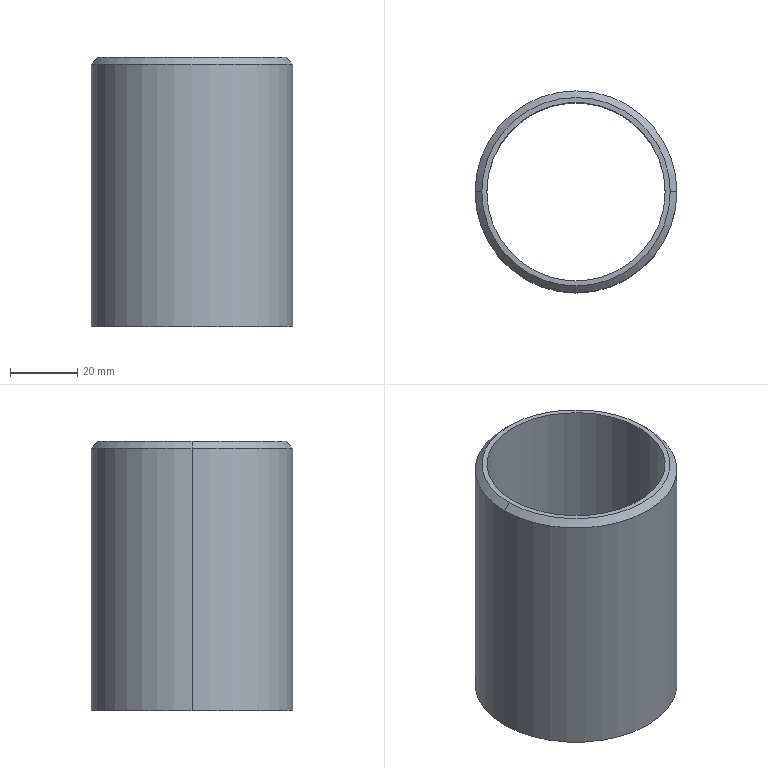Part | SolidWorks | features Chamfer 1, Extrusion 1 | 1 solid | 8 faces | box 60 x 60 x 80 mm | volume 49331 mm3 | cylinder 4 | cone 2 | plane 2 | commonest cylinder face diameters 53 x2 60 x2
STEP:
#1=CARTESIAN_POINT('',(28.,0.,80.));
#2=VERTEX_POINT('',#1);
#3=CARTESIAN_POINT('',(-28.,0.,80.));
#4=VERTEX_POINT('',#3);
#5=CARTESIAN_POINT('',(0.,0.,80.));
#6=DIRECTION('',(0.,0.,1.));
#7=DIRECTION('',(1.,0.,0.));
#8=AXIS2_PLACEMENT_3D('',#5,#6,#7);
#9=CIRCLE('',#8,28.);
#10=EDGE_CURVE('',#2,#4,#9,.T.);
#11=ORIENTED_EDGE('',*,*,#10,.F.);
#12=CARTESIAN_POINT('',(30.,0.,78.));
#13=VERTEX_POINT('',#12);
#14=CARTESIAN_POINT('',(28.,0.,80.));
#15=DIRECTION('',(0.7071,0.,-0.7071));
#16=VECTOR('',#15,1000.);
#17=LINE('',#14,#16);
#18=EDGE_CURVE('',#2,#13,#17,.T.);
#19=ORIENTED_EDGE('',*,*,#18,.T.);
#20=CARTESIAN_POINT('',(-30.,0.,78.));
#21=VERTEX_POINT('',#20);
#22=CARTESIAN_POINT('',(0.,0.,78.));
#23=DIRECTION('',(0.,0.,-1.));
#24=DIRECTION('',(1.,0.,0.));
#25=AXIS2_PLACEMENT_3D('',#22,#23,#24);
#26=CIRCLE('',#25,30.);
#27=EDGE_CURVE('',#21,#13,#26,.T.);
#28=ORIENTED_EDGE('',*,*,#27,.F.);
#29=CARTESIAN_POINT('',(-28.,0.,80.));
#30=DIRECTION('',(-0.7071,0.,-0.7071));
#31=VECTOR('',#30,1000.);
#32=LINE('',#29,#31);
#33=EDGE_CURVE('',#4,#21,#32,.T.);
#34=ORIENTED_EDGE('',*,*,#33,.F.);
#35=EDGE_LOOP('',(#11,#19,#28,#34));
#36=FACE_OUTER_BOUND('',#35,.T.);
#37=CARTESIAN_POINT('',(0.,0.,80.));
#38=DIRECTION('',(0.,0.,-1.));
#39=DIRECTION('',(-1.,0.,0.));
#40=AXIS2_PLACEMENT_3D('',#37,#38,#39);
#41=CONICAL_SURFACE('',#40,28.,0.7854);
#42=ADVANCED_FACE('',(#36),#41,.T.);
#43=CARTESIAN_POINT('',(-26.5,0.,80.));
#44=VERTEX_POINT('',#43);
#45=CARTESIAN_POINT('',(26.5,0.,80.));
#46=VERTEX_POINT('',#45);
#47=CARTESIAN_POINT('',(0.,0.,80.));
#48=DIRECTION('',(0.,0.,1.));
#49=DIRECTION('',(1.,0.,0.));
#50=AXIS2_PLACEMENT_3D('',#47,#48,#49);
#51=CIRCLE('',#50,26.5);
#52=EDGE_CURVE('',#44,#46,#51,.T.);
#53=ORIENTED_EDGE('',*,*,#52,.T.);
#54=CARTESIAN_POINT('',(26.5,0.,0.));
#55=VERTEX_POINT('',#54);
#56=CARTESIAN_POINT('',(26.5,0.,80.));
#57=DIRECTION('',(0.,0.,-1.));
#58=VECTOR('',#57,1000.);
#59=LINE('',#56,#58);
#60=EDGE_CURVE('',#46,#55,#59,.T.);
#61=ORIENTED_EDGE('',*,*,#60,.T.);
#62=CARTESIAN_POINT('',(-26.5,0.,0.));
#63=VERTEX_POINT('',#62);
#64=CARTESIAN_POINT('',(0.,0.,0.));
#65=DIRECTION('',(0.,0.,1.));
#66=DIRECTION('',(1.,0.,0.));
#67=AXIS2_PLACEMENT_3D('',#64,#65,#66);
#68=CIRCLE('',#67,26.5);
#69=EDGE_CURVE('',#63,#55,#68,.T.);
#70=ORIENTED_EDGE('',*,*,#69,.F.);
#71=CARTESIAN_POINT('',(-26.5,0.,80.));
#72=DIRECTION('',(0.,0.,-1.));
#73=VECTOR('',#72,1000.);
#74=LINE('',#71,#73);
#75=EDGE_CURVE('',#44,#63,#74,.T.);
#76=ORIENTED_EDGE('',*,*,#75,.F.);
#77=EDGE_LOOP('',(#53,#61,#70,#76));
#78=FACE_OUTER_BOUND('',#77,.T.);
#79=CARTESIAN_POINT('',(0.,0.,80.));
#80=DIRECTION('',(0.,0.,-1.));
#81=DIRECTION('',(-1.,0.,0.));
#82=AXIS2_PLACEMENT_3D('',#79,#80,#81);
#83=CYLINDRICAL_SURFACE('',#82,26.5);
#84=ADVANCED_FACE('',(#78),#83,.F.);
#85=ORIENTED_EDGE('',*,*,#27,.T.);
#86=CARTESIAN_POINT('',(30.,0.,0.));
#87=VERTEX_POINT('',#86);
#88=CARTESIAN_POINT('',(30.,0.,80.));
#89=DIRECTION('',(0.,0.,-1.));
#90=VECTOR('',#89,1000.);
#91=LINE('',#88,#90);
#92=EDGE_CURVE('',#13,#87,#91,.T.);
#93=ORIENTED_EDGE('',*,*,#92,.T.);
#94=CARTESIAN_POINT('',(-30.,0.,0.));
#95=VERTEX_POINT('',#94);
#96=CARTESIAN_POINT('',(0.,0.,0.));
#97=DIRECTION('',(0.,0.,1.));
#98=DIRECTION('',(1.,0.,0.));
#99=AXIS2_PLACEMENT_3D('',#96,#97,#98);
#100=CIRCLE('',#99,30.);
#101=EDGE_CURVE('',#87,#95,#100,.T.);
#102=ORIENTED_EDGE('',*,*,#101,.T.);
#103=CARTESIAN_POINT('',(-30.,0.,80.));
#104=DIRECTION('',(0.,0.,-1.));
#105=VECTOR('',#104,1000.);
#106=LINE('',#103,#105);
#107=EDGE_CURVE('',#21,#95,#106,.T.);
#108=ORIENTED_EDGE('',*,*,#107,.F.);
#109=EDGE_LOOP('',(#85,#93,#102,#108));
#110=FACE_OUTER_BOUND('',#109,.T.);
#111=CARTESIAN_POINT('',(0.,0.,80.));
#112=DIRECTION('',(0.,0.,-1.));
#113=DIRECTION('',(-1.,0.,0.));
#114=AXIS2_PLACEMENT_3D('',#111,#112,#113);
#115=CYLINDRICAL_SURFACE('',#114,30.);
#116=ADVANCED_FACE('',(#110),#115,.T.);
#117=CARTESIAN_POINT('',(0.,0.,80.));
#118=DIRECTION('',(0.,0.,1.));
#119=DIRECTION('',(1.,0.,0.));
#120=AXIS2_PLACEMENT_3D('',#117,#118,#119);
#121=CIRCLE('',#120,28.);
#122=EDGE_CURVE('',#4,#2,#121,.T.);
#123=ORIENTED_EDGE('',*,*,#122,.T.);
#124=ORIENTED_EDGE('',*,*,#10,.T.);
#125=EDGE_LOOP('',(#123,#124));
#126=FACE_OUTER_BOUND('',#125,.T.);
#127=ORIENTED_EDGE('',*,*,#52,.F.);
#128=CARTESIAN_POINT('',(0.,0.,80.));
#129=DIRECTION('',(0.,0.,1.));
#130=DIRECTION('',(1.,0.,0.));
#131=AXIS2_PLACEMENT_3D('',#128,#129,#130);
#132=CIRCLE('',#131,26.5);
#133=EDGE_CURVE('',#46,#44,#132,.T.);
#134=ORIENTED_EDGE('',*,*,#133,.F.);
#135=EDGE_LOOP('',(#127,#134));
#136=FACE_BOUND('',#135,.T.);
#137=CARTESIAN_POINT('',(0.,0.,80.));
#138=DIRECTION('',(0.,0.,1.));
#139=DIRECTION('',(1.,0.,0.));
#140=AXIS2_PLACEMENT_3D('',#137,#138,#139);
#141=PLANE('',#140);
#142=ADVANCED_FACE('',(#126,#136),#141,.T.);
#143=CARTESIAN_POINT('',(0.,0.,0.));
#144=DIRECTION('',(0.,0.,1.));
#145=DIRECTION('',(1.,0.,0.));
#146=AXIS2_PLACEMENT_3D('',#143,#144,#145);
#147=CIRCLE('',#146,30.);
#148=EDGE_CURVE('',#95,#87,#147,.T.);
#149=ORIENTED_EDGE('',*,*,#148,.F.);
#150=ORIENTED_EDGE('',*,*,#101,.F.);
#151=EDGE_LOOP('',(#149,#150));
#152=FACE_OUTER_BOUND('',#151,.T.);
#153=ORIENTED_EDGE('',*,*,#69,.T.);
#154=CARTESIAN_POINT('',(0.,0.,0.));
#155=DIRECTION('',(0.,0.,1.));
#156=DIRECTION('',(1.,0.,0.));
#157=AXIS2_PLACEMENT_3D('',#154,#155,#156);
#158=CIRCLE('',#157,26.5);
#159=EDGE_CURVE('',#55,#63,#158,.T.);
#160=ORIENTED_EDGE('',*,*,#159,.T.);
#161=EDGE_LOOP('',(#153,#160));
#162=FACE_BOUND('',#161,.T.);
#163=CARTESIAN_POINT('',(0.,0.,0.));
#164=DIRECTION('',(0.,0.,1.));
#165=DIRECTION('',(1.,0.,0.));
#166=AXIS2_PLACEMENT_3D('',#163,#164,#165);
#167=PLANE('',#166);
#168=ADVANCED_FACE('',(#152,#162),#167,.F.);
#169=ORIENTED_EDGE('',*,*,#92,.F.);
#170=CARTESIAN_POINT('',(0.,0.,78.));
#171=DIRECTION('',(0.,0.,-1.));
#172=DIRECTION('',(1.,0.,0.));
#173=AXIS2_PLACEMENT_3D('',#170,#171,#172);
#174=CIRCLE('',#173,30.);
#175=EDGE_CURVE('',#13,#21,#174,.T.);
#176=ORIENTED_EDGE('',*,*,#175,.T.);
#177=ORIENTED_EDGE('',*,*,#107,.T.);
#178=ORIENTED_EDGE('',*,*,#148,.T.);
#179=EDGE_LOOP('',(#169,#176,#177,#178));
#180=FACE_OUTER_BOUND('',#179,.T.);
#181=CARTESIAN_POINT('',(0.,0.,80.));
#182=DIRECTION('',(0.,0.,-1.));
#183=DIRECTION('',(-1.,0.,0.));
#184=AXIS2_PLACEMENT_3D('',#181,#182,#183);
#185=CYLINDRICAL_SURFACE('',#184,30.);
#186=ADVANCED_FACE('',(#180),#185,.T.);
#187=ORIENTED_EDGE('',*,*,#60,.F.);
#188=ORIENTED_EDGE('',*,*,#133,.T.);
#189=ORIENTED_EDGE('',*,*,#75,.T.);
#190=ORIENTED_EDGE('',*,*,#159,.F.);
#191=EDGE_LOOP('',(#187,#188,#189,#190));
#192=FACE_OUTER_BOUND('',#191,.T.);
#193=CARTESIAN_POINT('',(0.,0.,80.));
#194=DIRECTION('',(0.,0.,-1.));
#195=DIRECTION('',(-1.,0.,0.));
#196=AXIS2_PLACEMENT_3D('',#193,#194,#195);
#197=CYLINDRICAL_SURFACE('',#196,26.5);
#198=ADVANCED_FACE('',(#192),#197,.F.);
#199=ORIENTED_EDGE('',*,*,#18,.F.);
#200=ORIENTED_EDGE('',*,*,#122,.F.);
#201=ORIENTED_EDGE('',*,*,#33,.T.);
#202=ORIENTED_EDGE('',*,*,#175,.F.);
#203=EDGE_LOOP('',(#199,#200,#201,#202));
#204=FACE_OUTER_BOUND('',#203,.T.);
#205=CARTESIAN_POINT('',(0.,0.,80.));
#206=DIRECTION('',(0.,0.,-1.));
#207=DIRECTION('',(-1.,0.,0.));
#208=AXIS2_PLACEMENT_3D('',#205,#206,#207);
#209=CONICAL_SURFACE('',#208,28.,0.7854);
#210=ADVANCED_FACE('',(#204),#209,.T.);
#211=CLOSED_SHELL('',(#42,#84,#116,#142,#168,#186,#198,#210));
#212=MANIFOLD_SOLID_BREP('',#211);
#213=CARTESIAN_POINT('',(0.,0.,0.));
#214=DIRECTION('',(0.,0.,1.));
#215=DIRECTION('',(1.,0.,0.));
#216=AXIS2_PLACEMENT_3D('',#213,#214,#215);
#217=(LENGTH_UNIT()NAMED_UNIT(*)SI_UNIT(.MILLI.,.METRE.));
#218=UNCERTAINTY_MEASURE_WITH_UNIT(LENGTH_MEASURE(0.00001),#217,'','');
#219=(NAMED_UNIT(*)PLANE_ANGLE_UNIT()SI_UNIT($,.RADIAN.));
#220=(NAMED_UNIT(*)SI_UNIT($,.STERADIAN.)SOLID_ANGLE_UNIT());
#221=(GEOMETRIC_REPRESENTATION_CONTEXT(3)GLOBAL_UNCERTAINTY_ASSIGNED_CONTEXT((#218))GLOBAL_UNIT_ASSIGNED_CONTEXT((#217,#219,#220))REPRESENTATION_CONTEXT('',''));
#222=ADVANCED_BREP_SHAPE_REPRESENTATION('',(#212,#216),#221);